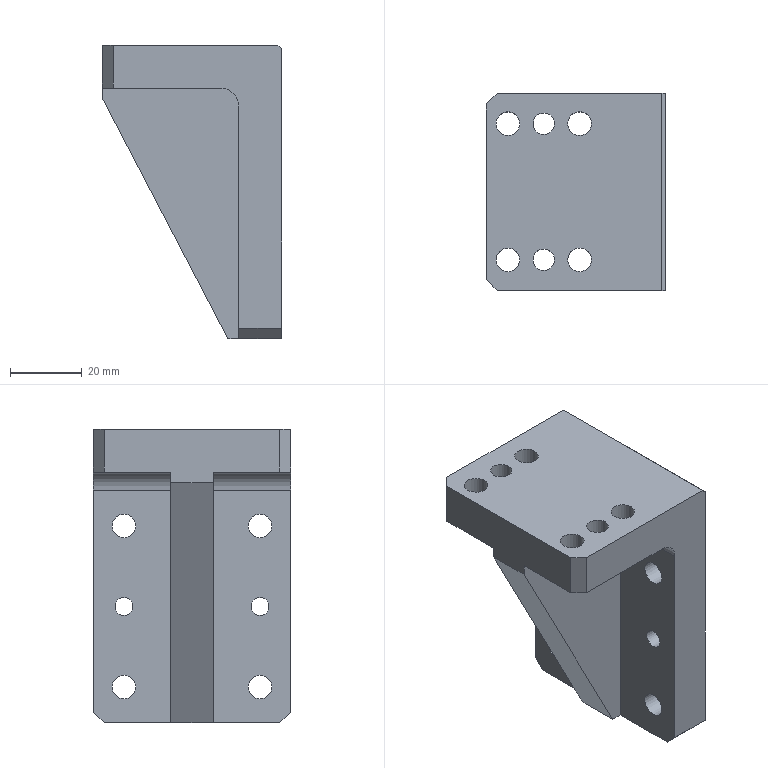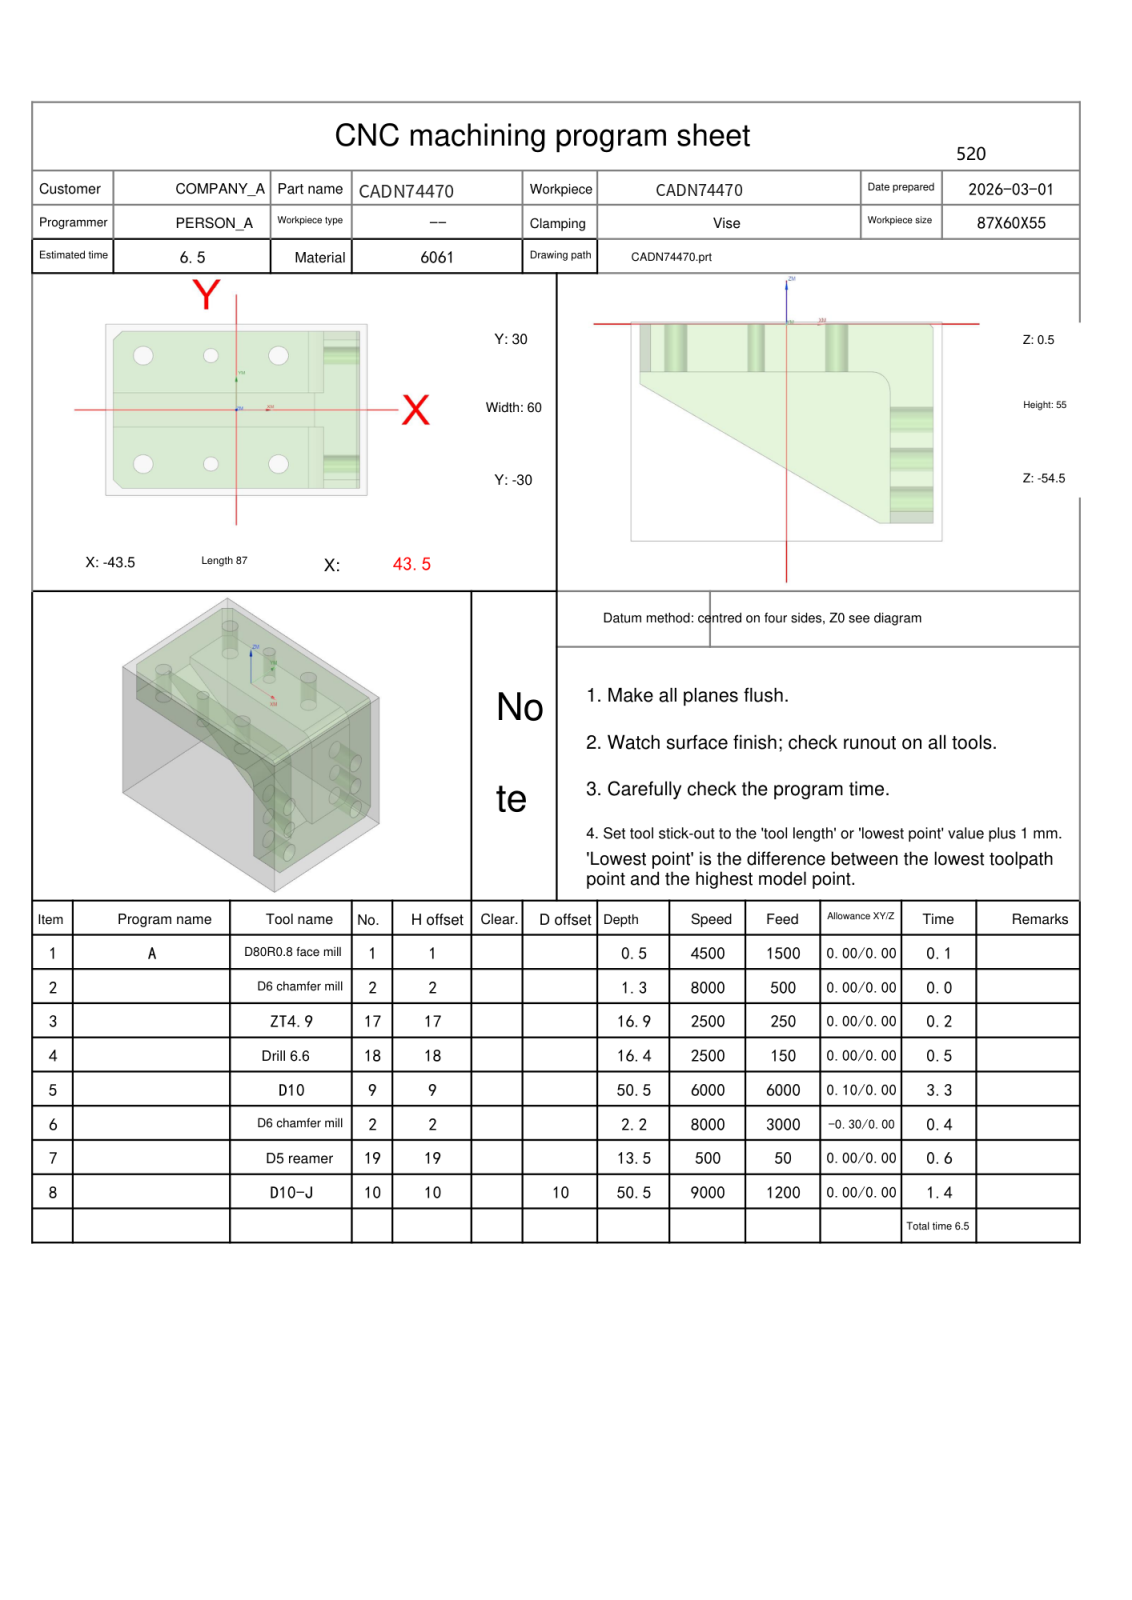NC program | NX | posted by the shop | part box 50 x 55 x 82 mm
Whole program:
%
O0001
(Machine time: 7.98 MIN)
(===Total Tool:7===)
(T1=D80R0.8 face mill D=80.  R=0.8  D-  H01 Z=-0.   )
(T2=D6 chamfer mill   D=6.   R=0.   D-  H02 Z=-1.7  )
(T17=ZT4.9  D=4.9  DR_a=120 D-  H17 Z=-16.41)
(T18=drill 6.6  D=6.6  DR_a=120 D-  H18 Z=-15.91)
(T9=D10     D=10.  R=0.   D-  H09 Z=-50.  )
(T19=D5 reamer   D=5.   DR_a=180 D-  H19 Z=-13.  )
(T10=D10-J  D=10.  R=0.   D10 H10 Z=-50.  )
G80 G90 G17 G49 G40
G91 G28 Z0
M01
N1 T01 M06
(D80R0.8 face mill  D=80. R=0.8 H=01 ce=0.00 di=0.00)
G00 G90 G54 X86. Y0.0 M03 S4500
G43 H01 Z50.
M08
Z2.
G01 Z0.0 F1500.
X81.
X-81.
X-86.
Z2.
G00 Z50.
G91 G28 Z0.0
M05
M09
G91 G28 Z0.0
M01
N2 T02 M06
(D6 chamfer mill  D=6. R=0. H=02 ce=0.00 di=0.00)
G00 G90 G54 X14. Y-19. M03 S8000
G43 H02 Z50.
M08
G98 G81 X14. Y-19. Z-.8 R1. F500.
X-8.5
X-31.
Y19.
X-8.5
X14.
G80
G00 Z50.
G91 G28 Z0.0
M05
M09
G91 G28 Z0.0
M01
N3 T17 M06
(ZT4.9 D=4.9 DR_a=120 H=17)
G00 G90 G54 X-8.5 Y-19. M03 S2500
G43 H17 Z50.
M08
G98 G83 X-8.5 Y-19. Z-16.415 R1. F250. Q2.
Y19.
G80
G00 Z50.
G91 G28 Z0.0
M05
M09
G91 G28 Z0.0
M01
N4 T18 M06
(drill 6.6 D=6.6 DR_a=120 H=18)
G00 G90 G54 X14. Y-19. M03 S2500
G43 H18 Z50.
M08
G98 G83 X14. Y-19. Z-15.905 R1. F150. Q3.
Y19.
X-31.
Y-19.
G80
G00 Z50.
G91 G28 Z0.0
M05
M09
G91 G28 Z0.0
M01
N5 T09 M06
(D10  D=10. R=0. H=09 ce=0.10 di=0.00)
G00 G90 G54 X1.081 Y-32.6 M03 S6000
G43 H09 Z50.
M08
Z.5
G01 X-38. Z.398 F6000.
G02 X-38.835 Y-32.531 Z.396 I0.0 J5.1
X-41.606 Y-31.106 Z.388 I.835 J5.031
G01 X-44.606 Y-28.106 Z.377
G02 X-46.1 Y-24.5 Z.366 I3.606 J3.606
G01 Y24.5 Z.238
G02 X-44.606 Y28.106 Z.228 I5.1 J0.0
G01 X-41.606 Y31.106 Z.217
G02 X-38. Y32.6 Z.206 I3.606 J-3.606
G01 X41. Z0.0
G02 X46.1 Y27.5 Z-.021 I0.0 J-5.1
G01 Y-27.5 Z-.164
G02 X41. Y-32.6 Z-.185 I-5.1 J0.0
G01 X-38. Z-.391
G02 X-38.835 Y-32.531 Z-.393 I0.0 J5.1
X-41.606 Y-31.106 Z-.401 I.835 J5.031
G01 X-44.606 Y-28.106 Z-.413
G02 X-46.1 Y-24.5 Z-.423 I3.606 J3.606
G01 Y24.5 Z-.551
G02 X-44.606 Y28.106 Z-.561 I5.1 J0.0
G01 X-41.606 Y31.106 Z-.572
G02 X-38. Y32.6 Z-.583 I3.606 J-3.606
G01 X41. Z-.789
G02 X46.1 Y27.5 Z-.81 I0.0 J-5.1
G01 Y-27.5 Z-.953
G02 X41. Y-32.6 Z-.974 I-5.1 J0.0
G01 X-38. Z-1.18
G02 X-38.835 Y-32.531 Z-1.182 I0.0 J5.1
X-41.606 Y-31.106 Z-1.191 I.835 J5.031
G01 X-44.606 Y-28.106 Z-1.202
G02 X-46.1 Y-24.5 Z-1.212 I3.606 J3.606
G01 Y24.5 Z-1.34
G02 X-44.606 Y28.106 Z-1.35 I5.1 J0.0
G01 X-41.606 Y31.106 Z-1.361
G02 X-38. Y32.6 Z-1.372 I3.606 J-3.606
G01 X41. Z-1.578
G02 X46.1 Y27.5 Z-1.599 I0.0 J-5.1
G01 Y-27.5 Z-1.742
G02 X41. Y-32.6 Z-1.763 I-5.1 J0.0
G01 X-38. Z-1.969
G02 X-38.835 Y-32.531 Z-1.971 I0.0 J5.1
X-41.606 Y-31.106 Z-1.98 I.835 J5.031
G01 X-44.606 Y-28.106 Z-1.991
G02 X-46.1 Y-24.5 Z-2.001 I3.606 J3.606
G01 Y24.5 Z-2.129
G02 X-44.606 Y28.106 Z-2.139 I5.1 J0.0
G01 X-41.606 Y31.106 Z-2.15
G02 X-38. Y32.6 Z-2.161 I3.606 J-3.606
G01 X41. Z-2.367
G02 X46.1 Y27.5 Z-2.388 I0.0 J-5.1
G01 Y-27.5 Z-2.531
G02 X41. Y-32.6 Z-2.552 I-5.1 J0.0
G01 X-38. Z-2.758
G02 X-38.835 Y-32.531 Z-2.76 I0.0 J5.1
X-41.606 Y-31.106 Z-2.769 I.835 J5.031
G01 X-44.606 Y-28.106 Z-2.78
G02 X-46.1 Y-24.5 Z-2.79 I3.606 J3.606
G01 Y24.5 Z-2.918
G02 X-44.606 Y28.106 Z-2.928 I5.1 J0.0
G01 X-41.606 Y31.106 Z-2.939
G02 X-38. Y32.6 Z-2.95 I3.606 J-3.606
G01 X41. Z-3.156
G02 X46.1 Y27.5 Z-3.177 I0.0 J-5.1
G01 Y-27.5 Z-3.32
G02 X41. Y-32.6 Z-3.341 I-5.1 J0.0
G01 X-38. Z-3.547
G02 X-38.835 Y-32.531 Z-3.549 I0.0 J5.1
X-41.606 Y-31.106 Z-3.558 I.835 J5.031
G01 X-44.606 Y-28.106 Z-3.569
G02 X-46.1 Y-24.5 Z-3.579 I3.606 J3.606
G01 Y24.5 Z-3.707
G02 X-44.606 Y28.106 Z-3.717 I5.1 J0.0
G01 X-41.606 Y31.106 Z-3.729
G02 X-38. Y32.6 Z-3.739 I3.606 J-3.606
G01 X41. Z-3.945
G02 X46.1 Y27.5 Z-3.966 I0.0 J-5.1
G01 Y-27.5 Z-4.109
G02 X41. Y-32.6 Z-4.13 I-5.1 J0.0
G01 X-38. Z-4.336
G02 X-38.835 Y-32.531 Z-4.338 I0.0 J5.1
X-41.606 Y-31.106 Z-4.347 I.835 J5.031
G01 X-44.606 Y-28.106 Z-4.358
G02 X-46.1 Y-24.5 Z-4.368 I3.606 J3.606
G01 Y24.5 Z-4.496
G02 X-44.606 Y28.106 Z-4.507 I5.1 J0.0
G01 X-41.606 Y31.106 Z-4.518
G02 X-38. Y32.6 Z-4.528 I3.606 J-3.606
G01 X41. Z-4.734
G02 X46.1 Y27.5 Z-4.755 I0.0 J-5.1
G01 Y-27.5 Z-4.898
G02 X41. Y-32.6 Z-4.919 I-5.1 J0.0
G01 X-38. Z-5.125
G02 X-38.835 Y-32.531 Z-5.128 I0.0 J5.1
X-41.606 Y-31.106 Z-5.136 I.835 J5.031
G01 X-44.606 Y-28.106 Z-5.147
G02 X-46.1 Y-24.5 Z-5.157 I3.606 J3.606
G01 Y24.5 Z-5.285
G02 X-44.606 Y28.106 Z-5.296 I5.1 J0.0
G01 X-41.606 Y31.106 Z-5.307
G02 X-38. Y32.6 Z-5.317 I3.606 J-3.606
G01 X41. Z-5.523
G02 X46.1 Y27.5 Z-5.544 I0.0 J-5.1
G01 Y-27.5 Z-5.687
G02 X41. Y-32.6 Z-5.708 I-5.1 J0.0
G01 X-38. Z-5.914
G02 X-38.835 Y-32.531 Z-5.917 I0.0 J5.1
X-41.606 Y-31.106 Z-5.925 I.835 J5.031
G01 X-44.606 Y-28.106 Z-5.936
G02 X-46.1 Y-24.5 Z-5.946 I3.606 J3.606
G01 Y24.5 Z-6.074
G02 X-44.606 Y28.106 Z-6.085 I5.1 J0.0
G01 X-41.606 Y31.106 Z-6.096
G02 X-38. Y32.6 Z-6.106 I3.606 J-3.606
G01 X41. Z-6.312
G02 X46.1 Y27.5 Z-6.333 I0.0 J-5.1
G01 Y-27.5 Z-6.477
G02 X41. Y-32.6 Z-6.497 I-5.1 J0.0
G01 X-38. Z-6.703
G02 X-38.835 Y-32.531 Z-6.706 I0.0 J5.1
X-41.606 Y-31.106 Z-6.714 I.835 J5.031
G01 X-44.606 Y-28.106 Z-6.725
G02 X-46.1 Y-24.5 Z-6.735 I3.606 J3.606
G01 Y24.5 Z-6.863
G02 X-44.606 Y28.106 Z-6.874 I5.1 J0.0
G01 X-41.606 Y31.106 Z-6.885
G02 X-38. Y32.6 Z-6.895 I3.606 J-3.606
G01 X41. Z-7.101
G02 X46.1 Y27.5 Z-7.122 I0.0 J-5.1
G01 Y-27.5 Z-7.266
G02 X41. Y-32.6 Z-7.287 I-5.1 J0.0
G01 X-38. Z-7.493
G02 X-38.835 Y-32.531 Z-7.495 I0.0 J5.1
X-41.606 Y-31.106 Z-7.503 I.835 J5.031
G01 X-44.606 Y-28.106 Z-7.514
G02 X-46.1 Y-24.5 Z-7.525 I3.606 J3.606
G01 Y24.5 Z-7.652
G02 X-44.606 Y28.106 Z-7.663 I5.1 J0.0
G01 X-41.606 Y31.106 Z-7.674
G02 X-38. Y32.6 Z-7.684 I3.606 J-3.606
G01 X41. Z-7.89
G02 X46.1 Y27.5 Z-7.911 I0.0 J-5.1
G01 Y-27.5 Z-8.055
G02 X41. Y-32.6 Z-8.076 I-5.1 J0.0
G01 X-38. Z-8.282
G02 X-38.835 Y-32.531 Z-8.284 I0.0 J5.1
X-41.606 Y-31.106 Z-8.292 I.835 J5.031
G01 X-44.606 Y-28.106 Z-8.303
G02 X-46.1 Y-24.5 Z-8.314 I3.606 J3.606
G01 Y24.5 Z-8.441
G02 X-44.606 Y28.106 Z-8.452 I5.1 J0.0
G01 X-41.606 Y31.106 Z-8.463
G02 X-38. Y32.6 Z-8.473 I3.606 J-3.606
G01 X41. Z-8.679
G02 X46.1 Y27.5 Z-8.7 I0.0 J-5.1
G01 Y-27.5 Z-8.844
G02 X41. Y-32.6 Z-8.865 I-5.1 J0.0
G01 X-38. Z-9.071
G02 X-38.835 Y-32.531 Z-9.073 I0.0 J5.1
X-41.606 Y-31.106 Z-9.081 I.835 J5.031
G01 X-44.606 Y-28.106 Z-9.092
G02 X-46.1 Y-24.5 Z-9.103 I3.606 J3.606
G01 Y24.5 Z-9.23
G02 X-44.606 Y28.106 Z-9.241 I5.1 J0.0
G01 X-41.606 Y31.106 Z-9.252
G02 X-38. Y32.6 Z-9.262 I3.606 J-3.606
G01 X41. Z-9.468
G02 X46.1 Y27.5 Z-9.489 I0.0 J-5.1
G01 Y-27.5 Z-9.633
G02 X41. Y-32.6 Z-9.654 I-5.1 J0.0
G01 X-38. Z-9.86
G02 X-38.835 Y-32.531 Z-9.862 I0.0 J5.1
X-41.606 Y-31.106 Z-9.87 I.835 J5.031
G01 X-44.606 Y-28.106 Z-9.881
G02 X-46.1 Y-24.5 Z-9.892 I3.606 J3.606
G01 Y24.5 Z-10.02
G02 X-44.606 Y28.106 Z-10.03 I5.1 J0.0
G01 X-41.606 Y31.106 Z-10.041
G02 X-38. Y32.6 Z-10.051 I3.606 J-3.606
G01 X41. Z-10.258
G02 X46.1 Y27.5 Z-10.278 I0.0 J-5.1
G01 Y-27.5 Z-10.422
G02 X41. Y-32.6 Z-10.443 I-5.1 J0.0
G01 X-38. Z-10.649
G02 X-38.835 Y-32.531 Z-10.651 I0.0 J5.1
X-41.606 Y-31.106 Z-10.659 I.835 J5.031
G01 X-44.606 Y-28.106 Z-10.67
G02 X-46.1 Y-24.5 Z-10.681 I3.606 J3.606
G01 Y24.5 Z-10.809
G02 X-44.606 Y28.106 Z-10.819 I5.1 J0.0
G01 X-41.606 Y31.106 Z-10.83
G02 X-38. Y32.6 Z-10.841 I3.606 J-3.606
G01 X41. Z-11.047
G02 X46.1 Y27.5 Z-11.067 I0.0 J-5.1
G01 Y-27.5 Z-11.211
G02 X41. Y-32.6 Z-11.232 I-5.1 J0.0
G01 X-38. Z-11.438
G02 X-38.835 Y-32.531 Z-11.44 I0.0 J5.1
X-41.606 Y-31.106 Z-11.448 I.835 J5.031
G01 X-44.606 Y-28.106 Z-11.459
G02 X-46.1 Y-24.5 Z-11.47 I3.606 J3.606
G01 Y24.5 Z-11.598
G02 X-44.606 Y28.106 Z-11.608 I5.1 J0.0
G01 X-41.606 Y31.106 Z-11.619
G02 X-38. Y32.6 Z-11.63 I3.606 J-3.606
G01 X41. Z-11.836
G02 X46.1 Y27.5 Z-11.857 I0.0 J-5.1
G01 Y-27.5 Z-12.
G02 X41. Y-32.6 Z-12.021 I-5.1 J0.0
G01 X-38. Z-12.227
G02 X-38.835 Y-32.531 Z-12.229 I0.0 J5.1
X-41.606 Y-31.106 Z-12.237 I.835 J5.031
G01 X-44.606 Y-28.106 Z-12.248
G02 X-46.1 Y-24.5 Z-12.259 I3.606 J3.606
G01 Y24.5 Z-12.387
G02 X-44.606 Y28.106 Z-12.397 I5.1 J0.0
G01 X-41.606 Y31.106 Z-12.408
G02 X-38. Y32.6 Z-12.419 I3.606 J-3.606
G01 X41. Z-12.625
G02 X46.1 Y27.5 Z-12.646 I0.0 J-5.1
G01 Y-27.5 Z-12.789
G02 X41. Y-32.6 Z-12.81 I-5.1 J0.0
G01 X-38. Z-13.016
G02 X-38.835 Y-32.531 Z-13.018 I0.0 J5.1
X-41.606 Y-31.106 Z-13.026 I.835 J5.031
G01 X-44.606 Y-28.106 Z-13.038
G02 X-46.1 Y-24.5 Z-13.048 I3.606 J3.606
G01 Y24.5 Z-13.176
G02 X-44.606 Y28.106 Z-13.186 I5.1 J0.0
G01 X-41.606 Y31.106 Z-13.197
G02 X-38. Y32.6 Z-13.208 I3.606 J-3.606
G01 X41. Z-13.414
G02 X46.1 Y27.5 Z-13.435 I0.0 J-5.1
G01 Y-27.5 Z-13.578
G02 X41. Y-32.6 Z-13.599 I-5.1 J0.0
G01 X-38. Z-13.805
G02 X-38.835 Y-32.531 Z-13.807 I0.0 J5.1
X-41.606 Y-31.106 Z-13.816 I.835 J5.031
G01 X-44.606 Y-28.106 Z-13.827
G02 X-46.1 Y-24.5 Z-13.837 I3.606 J3.606
G01 Y24.5 Z-13.965
G02 X-44.606 Y28.106 Z-13.975 I5.1 J0.0
G01 X-41.606 Y31.106 Z-13.986
G02 X-38. Y32.6 Z-13.997 I3.606 J-3.606
G01 X41. Z-14.203
G02 X46.1 Y27.5 Z-14.224 I0.0 J-5.1
G01 Y-27.5 Z-14.367
G02 X41. Y-32.6 Z-14.388 I-5.1 J0.0
G01 X-38. Z-14.594
G02 X-38.835 Y-32.531 Z-14.596 I0.0 J5.1
X-41.606 Y-31.106 Z-14.605 I.835 J5.031
G01 X-44.606 Y-28.106 Z-14.616
G02 X-46.1 Y-24.5 Z-14.626 I3.606 J3.606
G01 Y24.5 Z-14.754
G02 X-44.606 Y28.106 Z-14.764 I5.1 J0.0
G01 X-41.606 Y31.106 Z-14.775
G02 X-38. Y32.6 Z-14.786 I3.606 J-3.606
G01 X41. Z-14.992
G02 X46.1 Y27.5 Z-15.013 I0.0 J-5.1
G01 Y-27.5 Z-15.156
G02 X41. Y-32.6 Z-15.177 I-5.1 J0.0
G01 X-38. Z-15.383
G02 X-38.835 Y-32.531 Z-15.385 I0.0 J5.1
X-41.606 Y-31.106 Z-15.394 I.835 J5.031
G01 X-44.606 Y-28.106 Z-15.405
G02 X-46.1 Y-24.5 Z-15.415 I3.606 J3.606
G01 Y24.5 Z-15.543
G02 X-44.606 Y28.106 Z-15.553 I5.1 J0.0
G01 X-41.606 Y31.106 Z-15.564
G02 X-38. Y32.6 Z-15.575 I3.606 J-3.606
G01 X41. Z-15.781
G02 X46.1 Y27.5 Z-15.802 I0.0 J-5.1
G01 Y-27.5 Z-15.945
G02 X41. Y-32.6 Z-15.966 I-5.1 J0.0
G01 X-38. Z-16.172
G02 X-38.835 Y-32.531 Z-16.174 I0.0 J5.1
X-41.606 Y-31.106 Z-16.183 I.835 J5.031
G01 X-44.606 Y-28.106 Z-16.194
G02 X-46.1 Y-24.5 Z-16.204 I3.606 J3.606
G01 Y24.5 Z-16.332
G02 X-44.606 Y28.106 Z-16.342 I5.1 J0.0
G01 X-41.606 Y31.106 Z-16.354
G02 X-38. Y32.6 Z-16.364 I3.606 J-3.606
G01 X41. Z-16.57
G02 X46.1 Y27.5 Z-16.591 I0.0 J-5.1
G01 Y-27.5 Z-16.734
G02 X41. Y-32.6 Z-16.755 I-5.1 J0.0
G01 X-38. Z-16.961
G02 X-38.835 Y-32.531 Z-16.963 I0.0 J5.1
X-41.606 Y-31.106 Z-16.972 I.835 J5.031
G01 X-44.606 Y-28.106 Z-16.983
G02 X-46.1 Y-24.5 Z-16.993 I3.606 J3.606
G01 Y24.5 Z-17.121
G02 X-44.606 Y28.106 Z-17.132 I5.1 J0.0
G01 X-41.606 Y31.106 Z-17.143
G02 X-38. Y32.6 Z-17.153 I3.606 J-3.606
G01 X41. Z-17.359
G02 X46.1 Y27.5 Z-17.38 I0.0 J-5.1
G01 Y-27.5 Z-17.523
G02 X41. Y-32.6 Z-17.544 I-5.1 J0.0
G01 X-38. Z-17.75
G02 X-38.835 Y-32.531 Z-17.753 I0.0 J5.1
X-41.606 Y-31.106 Z-17.761 I.835 J5.031
G01 X-44.606 Y-28.106 Z-17.772
G02 X-46.1 Y-24.5 Z-17.782 I3.606 J3.606
G01 Y24.5 Z-17.91
G02 X-44.606 Y28.106 Z-17.921 I5.1 J0.0
G01 X-41.606 Y31.106 Z-17.932
G02 X-38. Y32.6 Z-17.942 I3.606 J-3.606
G01 X41. Z-18.148
G02 X46.1 Y27.5 Z-18.169 I0.0 J-5.1
G01 Y-27.5 Z-18.312
G02 X41. Y-32.6 Z-18.333 I-5.1 J0.0
G01 X-38. Z-18.539
G02 X-38.835 Y-32.531 Z-18.542 I0.0 J5.1
X-41.606 Y-31.106 Z-18.55 I.835 J5.031
G01 X-44.606 Y-28.106 Z-18.561
G02 X-46.1 Y-24.5 Z-18.571 I3.606 J3.606
G01 Y24.5 Z-18.699
G02 X-44.606 Y28.106 Z-18.71 I5.1 J0.0
G01 X-41.606 Y31.106 Z-18.721
G02 X-38. Y32.6 Z-18.731 I3.606 J-3.606
G01 X41. Z-18.937
G02 X46.1 Y27.5 Z-18.958 I0.0 J-5.1
G01 Y-27.5 Z-19.102
G02 X41. Y-32.6 Z-19.122 I-5.1 J0.0
G01 X-38. Z-19.328
G02 X-38.835 Y-32.531 Z-19.331 I0.0 J5.1
X-41.606 Y-31.106 Z-19.339 I.835 J5.031
G01 X-44.606 Y-28.106 Z-19.35
G02 X-46.1 Y-24.5 Z-19.36 I3.606 J3.606
G01 Y24.5 Z-19.488
G02 X-44.606 Y28.106 Z-19.499 I5.1 J0.0
G01 X-41.606 Y31.106 Z-19.51
G02 X-38. Y32.6 Z-19.52 I3.606 J-3.606
G01 X41. Z-19.726
G02 X46.1 Y27.5 Z-19.747 I0.0 J-5.1
G01 Y-27.5 Z-19.891
G02 X41. Y-32.6 Z-19.912 I-5.1 J0.0
G01 X-38. Z-20.118
G02 X-38.835 Y-32.531 Z-20.12 I0.0 J5.1
X-41.606 Y-31.106 Z-20.128 I.835 J5.031
G01 X-44.606 Y-28.106 Z-20.139
G02 X-46.1 Y-24.5 Z-20.15 I3.606 J3.606
G01 Y24.5 Z-20.277
G02 X-44.606 Y28.106 Z-20.288 I5.1 J0.0
G01 X-41.606 Y31.106 Z-20.299
G02 X-38. Y32.6 Z-20.309 I3.606 J-3.606
G01 X41. Z-20.515
G02 X46.1 Y27.5 Z-20.536 I0.0 J-5.1
G01 Y-27.5 Z-20.68
G02 X41. Y-32.6 Z-20.701 I-5.1 J0.0
G01 X-38. Z-20.907
G02 X-38.835 Y-32.531 Z-20.909 I0.0 J5.1
X-41.606 Y-31.106 Z-20.917 I.835 J5.031
G01 X-44.606 Y-28.106 Z-20.928
G02 X-46.1 Y-24.5 Z-20.939 I3.606 J3.606
G01 Y24.5 Z-21.066
G02 X-44.606 Y28.106 Z-21.077 I5.1 J0.0
G01 X-41.606 Y31.106 Z-21.088
G02 X-38. Y32.6 Z-21.098 I3.606 J-3.606
G01 X41. Z-21.304
G02 X46.1 Y27.5 Z-21.325 I0.0 J-5.1
G01 Y-27.5 Z-21.469
G02 X41. Y-32.6 Z-21.49 I-5.1 J0.0
G01 X-38. Z-21.696
G02 X-38.835 Y-32.531 Z-21.698 I0.0 J5.1
X-41.606 Y-31.106 Z-21.706 I.835 J5.031
G01 X-44.606 Y-28.106 Z-21.717
G02 X-46.1 Y-24.5 Z-21.728 I3.606 J3.606
G01 Y24.5 Z-21.855
G02 X-44.606 Y28.106 Z-21.866 I5.1 J0.0
G01 X-41.606 Y31.106 Z-21.877
G02 X-38. Y32.6 Z-21.887 I3.606 J-3.606
G01 X41. Z-22.093
G02 X46.1 Y27.5 Z-22.114 I0.0 J-5.1
G01 Y-27.5 Z-22.258
G02 X41. Y-32.6 Z-22.279 I-5.1 J0.0
G01 X-38. Z-22.485
G02 X-38.835 Y-32.531 Z-22.487 I0.0 J5.1
X-41.606 Y-31.106 Z-22.495 I.835 J5.031
G01 X-44.606 Y-28.106 Z-22.506
G02 X-46.1 Y-24.5 Z-22.517 I3.606 J3.606
G01 Y24.5 Z-22.645
G02 X-44.606 Y28.106 Z-22.655 I5.1 J0.0
G01 X-41.606 Y31.106 Z-22.666
G02 X-38. Y32.6 Z-22.676 I3.606 J-3.606
G01 X41. Z-22.883
G02 X46.1 Y27.5 Z-22.903 I0.0 J-5.1
G01 Y-27.5 Z-23.047
G02 X41. Y-32.6 Z-23.068 I-5.1 J0.0
G01 X-38. Z-23.274
G02 X-38.835 Y-32.531 Z-23.276 I0.0 J5.1
X-41.606 Y-31.106 Z-23.284 I.835 J5.031
G01 X-44.606 Y-28.106 Z-23.295
G02 X-46.1 Y-24.5 Z-23.306 I3.606 J3.606
G01 Y24.5 Z-23.434
G02 X-44.606 Y28.106 Z-23.444 I5.1 J0.0
G01 X-41.606 Y31.106 Z-23.455
G02 X-38. Y32.6 Z-23.466 I3.606 J-3.606
G01 X41. Z-23.672
G02 X46.1 Y27.5 Z-23.692 I0.0 J-5.1
G01 Y-27.5 Z-23.836
G02 X41. Y-32.6 Z-23.857 I-5.1 J0.0
G01 X-38. Z-24.063
G02 X-38.835 Y-32.531 Z-24.065 I0.0 J5.1
X-41.606 Y-31.106 Z-24.073 I.835 J5.031
G01 X-44.606 Y-28.106 Z-24.084
G02 X-46.1 Y-24.5 Z-24.095 I3.606 J3.606
G01 Y24.5 Z-24.223
G02 X-44.606 Y28.106 Z-24.233 I5.1 J0.0
G01 X-41.606 Y31.106 Z-24.244
G02 X-38. Y32.6 Z-24.255 I3.606 J-3.606
G01 X41. Z-24.461
G02 X46.1 Y27.5 Z-24.482 I0.0 J-5.1
G01 Y-27.5 Z-24.625
G02 X41. Y-32.6 Z-24.646 I-5.1 J0.0
G01 X-38. Z-24.852
G02 X-38.835 Y-32.531 Z-24.854 I0.0 J5.1
X-41.606 Y-31.106 Z-24.862 I.835 J5.031
G01 X-44.606 Y-28.106 Z-24.873
G02 X-46.1 Y-24.5 Z-24.884 I3.606 J3.606
G01 Y24.5 Z-25.012
G02 X-44.606 Y28.106 Z-25.022 I5.1 J0.0
G01 X-41.606 Y31.106 Z-25.033
G02 X-38. Y32.6 Z-25.044 I3.606 J-3.606
G01 X41. Z-25.25
G02 X46.1 Y27.5 Z-25.271 I0.0 J-5.1
G01 Y-27.5 Z-25.414
G02 X41. Y-32.6 Z-25.435 I-5.1 J0.0
G01 X-38. Z-25.641
G02 X-38.835 Y-32.531 Z-25.643 I0.0 J5.1
X-41.606 Y-31.106 Z-25.651 I.835 J5.031
G01 X-44.606 Y-28.106 Z-25.663
G02 X-46.1 Y-24.5 Z-25.673 I3.606 J3.606
G01 Y24.5 Z-25.801
G02 X-44.606 Y28.106 Z-25.811 I5.1 J0.0
G01 X-41.606 Y31.106 Z-25.822
G02 X-38. Y32.6 Z-25.833 I3.606 J-3.606
G01 X41. Z-26.039
G02 X46.1 Y27.5 Z-26.06 I0.0 J-5.1
G01 Y-27.5 Z-26.203
G02 X41. Y-32.6 Z-26.224 I-5.1 J0.0
G01 X-38. Z-26.43
G02 X-38.835 Y-32.531 Z-26.432 I0.0 J5.1
X-41.606 Y-31.106 Z-26.441 I.835 J5.031
G01 X-44.606 Y-28.106 Z-26.452
G02 X-46.1 Y-24.5 Z-26.462 I3.606 J3.606
G01 Y24.5 Z-26.59
G02 X-44.606 Y28.106 Z-26.6 I5.1 J0.0
G01 X-41.606 Y31.106 Z-26.611
G02 X-38. Y32.6 Z-26.622 I3.606 J-3.606
G01 X41. Z-26.828
G02 X46.1 Y27.5 Z-26.849 I0.0 J-5.1
G01 Y-27.5 Z-26.992
G02 X41. Y-32.6 Z-27.013 I-5.1 J0.0
G01 X-38. Z-27.219
G02 X-38.835 Y-32.531 Z-27.221 I0.0 J5.1
X-41.606 Y-31.106 Z-27.23 I.835 J5.031
G01 X-44.606 Y-28.106 Z-27.241
G02 X-46.1 Y-24.5 Z-27.251 I3.606 J3.606
G01 Y24.5 Z-27.379
G02 X-44.606 Y28.106 Z-27.389 I5.1 J0.0
G01 X-41.606 Y31.106 Z-27.4
G02 X-38. Y32.6 Z-27.411 I3.606 J-3.606
G01 X41. Z-27.617
G02 X46.1 Y27.5 Z-27.638 I0.0 J-5.1
G01 Y-27.5 Z-27.781
G02 X41. Y-32.6 Z-27.802 I-5.1 J0.0
G01 X-38. Z-28.008
G02 X-38.835 Y-32.531 Z-28.01 I0.0 J5.1
X-41.606 Y-31.106 Z-28.019 I.835 J5.031
G01 X-44.606 Y-28.106 Z-28.03
G02 X-46.1 Y-24.5 Z-28.04 I3.606 J3.606
G01 Y24.5 Z-28.168
G02 X-44.606 Y28.106 Z-28.178 I5.1 J0.0
G01 X-41.606 Y31.106 Z-28.189
G02 X-38. Y32.6 Z-28.2 I3.606 J-3.606
G01 X41. Z-28.406
G02 X46.1 Y27.5 Z-28.427 I0.0 J-5.1
G01 Y-27.5 Z-28.57
G02 X41. Y-32.6 Z-28.591 I-5.1 J0.0
G01 X-38. Z-28.797
G02 X-38.835 Y-32.531 Z-28.799 I0.0 J5.1
X-41.606 Y-31.106 Z-28.808 I.835 J5.031
G01 X-44.606 Y-28.106 Z-28.819
G02 X-46.1 Y-24.5 Z-28.829 I3.606 J3.606
G01 Y24.5 Z-28.957
G02 X-44.606 Y28.106 Z-28.967 I5.1 J0.0
G01 X-41.606 Y31.106 Z-28.979
G02 X-38. Y32.6 Z-28.989 I3.606 J-3.606
G01 X41. Z-29.195
G02 X46.1 Y27.5 Z-29.216 I0.0 J-5.1
G01 Y-27.5 Z-29.359
G02 X41. Y-32.6 Z-29.38 I-5.1 J0.0
G01 X-38. Z-29.586
G02 X-38.835 Y-32.531 Z-29.588 I0.0 J5.1
X-41.606 Y-31.106 Z-29.597 I.835 J5.031
G01 X-44.606 Y-28.106 Z-29.608
G02 X-46.1 Y-24.5 Z-29.618 I3.606 J3.606
G01 Y24.5 Z-29.746
G02 X-44.606 Y28.106 Z-29.757 I5.1 J0.0
G01 X-41.606 Y31.106 Z-29.768
G02 X-38. Y32.6 Z-29.778 I3.606 J-3.606
G01 X41. Z-29.984
G02 X46.1 Y27.5 Z-30.005 I0.0 J-5.1
G01 Y-27.5 Z-30.148
G02 X41. Y-32.6 Z-30.169 I-5.1 J0.0
G01 X-38. Z-30.375
G02 X-38.835 Y-32.531 Z-30.378 I0.0 J5.1
X-41.606 Y-31.106 Z-30.386 I.835 J5.031
G01 X-44.606 Y-28.106 Z-30.397
G02 X-46.1 Y-24.5 Z-30.407 I3.606 J3.606
G01 Y24.5 Z-30.535
G02 X-44.606 Y28.106 Z-30.546 I5.1 J0.0
G01 X-41.606 Y31.106 Z-30.557
G02 X-38. Y32.6 Z-30.567 I3.606 J-3.606
G01 X41. Z-30.773
G02 X46.1 Y27.5 Z-30.794 I0.0 J-5.1
G01 Y-27.5 Z-30.937
G02 X41. Y-32.6 Z-30.958 I-5.1 J0.0
G01 X-38. Z-31.164
G02 X-38.835 Y-32.531 Z-31.167 I0.0 J5.1
X-41.606 Y-31.106 Z-31.175 I.835 J5.031
G01 X-44.606 Y-28.106 Z-31.186
G02 X-46.1 Y-24.5 Z-31.196 I3.606 J3.606
G01 Y24.5 Z-31.324
G02 X-44.606 Y28.106 Z-31.335 I5.1 J0.0
G01 X-41.606 Y31.106 Z-31.346
G02 X-38. Y32.6 Z-31.356 I3.606 J-3.606
G01 X41. Z-31.562
G02 X46.1 Y27.5 Z-31.583 I0.0 J-5.1
G01 Y-27.5 Z-31.727
G02 X41. Y-32.6 Z-31.747 I-5.1 J0.0
G01 X-38. Z-31.953
G02 X-38.835 Y-32.531 Z-31.956 I0.0 J5.1
X-41.606 Y-31.106 Z-31.964 I.835 J5.031
G01 X-44.606 Y-28.106 Z-31.975
G02 X-46.1 Y-24.5 Z-31.985 I3.606 J3.606
G01 Y24.5 Z-32.113
G02 X-44.606 Y28.106 Z-32.124 I5.1 J0.0
G01 X-41.606 Y31.106 Z-32.135
G02 X-38. Y32.6 Z-32.145 I3.606 J-3.606
G01 X41. Z-32.351
G02 X46.1 Y27.5 Z-32.372 I0.0 J-5.1
G01 Y-27.5 Z-32.516
G02 X41. Y-32.6 Z-32.537 I-5.1 J0.0
G01 X-38. Z-32.743
G02 X-38.835 Y-32.531 Z-32.745 I0.0 J5.1
X-41.606 Y-31.106 Z-32.753 I.835 J5.031
G01 X-44.606 Y-28.106 Z-32.764
G02 X-46.1 Y-24.5 Z-32.775 I3.606 J3.606
G01 Y24.5 Z-32.902
G02 X-44.606 Y28.106 Z-32.913 I5.1 J0.0
G01 X-41.606 Y31.106 Z-32.924
G02 X-38. Y32.6 Z-32.934 I3.606 J-3.606
G01 X41. Z-33.14
G02 X46.1 Y27.5 Z-33.161 I0.0 J-5.1
G01 Y-27.5 Z-33.305
G02 X41. Y-32.6 Z-33.326 I-5.1 J0.0
G01 X-38. Z-33.532
G02 X-38.835 Y-32.531 Z-33.534 I0.0 J5.1
X-41.606 Y-31.106 Z-33.542 I.835 J5.031
G01 X-44.606 Y-28.106 Z-33.553
G02 X-46.1 Y-24.5 Z-33.564 I3.606 J3.606
G01 Y24.5 Z-33.691
G02 X-44.606 Y28.106 Z-33.702 I5.1 J0.0
G01 X-41.606 Y31.106 Z-33.713
G02 X-38. Y32.6 Z-33.723 I3.606 J-3.606
G01 X41. Z-33.929
G02 X46.1 Y27.5 Z-33.95 I0.0 J-5.1
G01 Y-27.5 Z-34.094
G02 X41. Y-32.6 Z-34.115 I-5.1 J0.0
G01 X-38. Z-34.321
G02 X-38.835 Y-32.531 Z-34.323 I0.0 J5.1
X-41.606 Y-31.106 Z-34.331 I.835 J5.031
G01 X-44.606 Y-28.106 Z-34.342
G02 X-46.1 Y-24.5 Z-34.353 I3.606 J3.606
G01 Y24.5 Z-34.48
G02 X-44.606 Y28.106 Z-34.491 I5.1 J0.0
G01 X-41.606 Y31.106 Z-34.502
G02 X-38. Y32.6 Z-34.512 I3.606 J-3.606
G01 X41. Z-34.718
G02 X46.1 Y27.5 Z-34.739 I0.0 J-5.1
G01 Y-27.5 Z-34.883
G02 X41. Y-32.6 Z-34.904 I-5.1 J0.0
G01 X-38. Z-35.11
G02 X-38.835 Y-32.531 Z-35.112 I0.0 J5.1
X-41.606 Y-31.106 Z-35.12 I.835 J5.031
G01 X-44.606 Y-28.106 Z-35.131
G02 X-46.1 Y-24.5 Z-35.142 I3.606 J3.606
G01 Y24.5 Z-35.27
G02 X-44.606 Y28.106 Z-35.28 I5.1 J0.0
G01 X-41.606 Y31.106 Z-35.291
G02 X-38. Y32.6 Z-35.301 I3.606 J-3.606
G01 X41. Z-35.508
G02 X46.1 Y27.5 Z-35.528 I0.0 J-5.1
G01 Y-27.5 Z-35.672
G02 X41. Y-32.6 Z-35.693 I-5.1 J0.0
G01 X-38. Z-35.899
G02 X-38.835 Y-32.531 Z-35.901 I0.0 J5.1
X-41.606 Y-31.106 Z-35.909 I.835 J5.031
G01 X-44.606 Y-28.106 Z-35.92
G02 X-46.1 Y-24.5 Z-35.931 I3.606 J3.606
G01 Y24.5 Z-36.059
G02 X-44.606 Y28.106 Z-36.069 I5.1 J0.0
G01 X-41.606 Y31.106 Z-36.08
G02 X-38. Y32.6 Z-36.091 I3.606 J-3.606
G01 X41. Z-36.297
G02 X46.1 Y27.5 Z-36.317 I0.0 J-5.1
G01 Y-27.5 Z-36.461
G02 X41. Y-32.6 Z-36.482 I-5.1 J0.0
G01 X-38. Z-36.688
G02 X-38.835 Y-32.531 Z-36.69 I0.0 J5.1
X-41.606 Y-31.106 Z-36.698 I.835 J5.031
G01 X-44.606 Y-28.106 Z-36.709
G02 X-46.1 Y-24.5 Z-36.72 I3.606 J3.606
G01 Y24.5 Z-36.848
G02 X-44.606 Y28.106 Z-36.858 I5.1 J0.0
G01 X-41.606 Y31.106 Z-36.869
G02 X-38. Y32.6 Z-36.88 I3.606 J-3.606
G01 X41. Z-37.086
G02 X46.1 Y27.5 Z-37.107 I0.0 J-5.1
G01 Y-27.5 Z-37.25
G02 X41. Y-32.6 Z-37.271 I-5.1 J0.0
G01 X-38. Z-37.477
G02 X-38.835 Y-32.531 Z-37.479 I0.0 J5.1
X-41.606 Y-31.106 Z-37.487 I.835 J5.031
G01 X-44.606 Y-28.106 Z-37.498
G02 X-46.1 Y-24.5 Z-37.509 I3.606 J3.606
G01 Y24.5 Z-37.637
G02 X-44.606 Y28.106 Z-37.647 I5.1 J0.0
G01 X-41.606 Y31.106 Z-37.658
G02 X-38. Y32.6 Z-37.669 I3.606 J-3.606
G01 X41. Z-37.875
G02 X46.1 Y27.5 Z-37.896 I0.0 J-5.1
G01 Y-27.5 Z-38.039
G02 X41. Y-32.6 Z-38.06 I-5.1 J0.0
G01 X-38. Z-38.266
G02 X-38.835 Y-32.531 Z-38.268 I0.0 J5.1
X-41.606 Y-31.106 Z-38.276 I.835 J5.031
G01 X-44.606 Y-28.106 Z-38.288
G02 X-46.1 Y-24.5 Z-38.298 I3.606 J3.606
G01 Y24.5 Z-38.426
G02 X-44.606 Y28.106 Z-38.436 I5.1 J0.0
G01 X-41.606 Y31.106 Z-38.447
G02 X-38. Y32.6 Z-38.458 I3.606 J-3.606
G01 X41. Z-38.664
G02 X46.1 Y27.5 Z-38.685 I0.0 J-5.1
G01 Y-27.5 Z-38.828
G02 X41. Y-32.6 Z-38.849 I-5.1 J0.0
G01 X-38. Z-39.055
G02 X-38.835 Y-32.531 Z-39.057 I0.0 J5.1
X-41.606 Y-31.106 Z-39.066 I.835 J5.031
G01 X-44.606 Y-28.106 Z-39.077
G02 X-46.1 Y-24.5 Z-39.087 I3.606 J3.606
G01 Y24.5 Z-39.215
G02 X-44.606 Y28.106 Z-39.225 I5.1 J0.0
G01 X-41.606 Y31.106 Z-39.236
G02 X-38. Y32.6 Z-39.247 I3.606 J-3.606
G01 X41. Z-39.453
G02 X46.1 Y27.5 Z-39.474 I0.0 J-5.1
G01 Y-27.5 Z-39.617
G02 X41. Y-32.6 Z-39.638 I-5.1 J0.0
G01 X-38. Z-39.844
G02 X-38.835 Y-32.531 Z-39.846 I0.0 J5.1
X-41.606 Y-31.106 Z-39.855 I.835 J5.031
G01 X-44.606 Y-28.106 Z-39.866
G02 X-46.1 Y-24.5 Z-39.876 I3.606 J3.606
G01 Y24.5 Z-40.004
G02 X-44.606 Y28.106 Z-40.014 I5.1 J0.0
G01 X-41.606 Y31.106 Z-40.025
G02 X-38. Y32.6 Z-40.036 I3.606 J-3.606
G01 X41. Z-40.242
G02 X46.1 Y27.5 Z-40.263 I0.0 J-5.1
G01 Y-27.5 Z-40.406
G02 X41. Y-32.6 Z-40.427 I-5.1 J0.0
G01 X-38. Z-40.633
G02 X-38.835 Y-32.531 Z-40.635 I0.0 J5.1
X-41.606 Y-31.106 Z-40.644 I.835 J5.031
G01 X-44.606 Y-28.106 Z-40.655
G02 X-46.1 Y-24.5 Z-40.665 I3.606 J3.606
G01 Y24.5 Z-40.793
G02 X-44.606 Y28.106 Z-40.803 I5.1 J0.0
G01 X-41.606 Y31.106 Z-40.814
G02 X-38. Y32.6 Z-40.825 I3.606 J-3.606
G01 X41. Z-41.031
G02 X46.1 Y27.5 Z-41.052 I0.0 J-5.1
G01 Y-27.5 Z-41.195
G02 X41. Y-32.6 Z-41.216 I-5.1 J0.0
G01 X-38. Z-41.422
G02 X-38.835 Y-32.531 Z-41.424 I0.0 J5.1
X-41.606 Y-31.106 Z-41.433 I.835 J5.031
G01 X-44.606 Y-28.106 Z-41.444
G02 X-46.1 Y-24.5 Z-41.454 I3.606 J3.606
G01 Y24.5 Z-41.582
G02 X-44.606 Y28.106 Z-41.592 I5.1 J0.0
G01 X-41.606 Y31.106 Z-41.604
G02 X-38. Y32.6 Z-41.614 I3.606 J-3.606
G01 X41. Z-41.82
G02 X46.1 Y27.5 Z-41.841 I0.0 J-5.1
G01 Y-27.5 Z-41.984
G02 X41. Y-32.6 Z-42.005 I-5.1 J0.0
G01 X-38. Z-42.211
G02 X-38.835 Y-32.531 Z-42.213 I0.0 J5.1
X-41.606 Y-31.106 Z-42.222 I.835 J5.031
G01 X-44.606 Y-28.106 Z-42.233
G02 X-46.1 Y-24.5 Z-42.243 I3.606 J3.606
G01 Y24.5 Z-42.371
G02 X-44.606 Y28.106 Z-42.382 I5.1 J0.0
G01 X-41.606 Y31.106 Z-42.393
G02 X-38. Y32.6 Z-42.403 I3.606 J-3.606
G01 X41. Z-42.609
G02 X46.1 Y27.5 Z-42.63 I0.0 J-5.1
G01 Y-27.5 Z-42.773
G02 X41. Y-32.6 Z-42.794 I-5.1 J0.0
G01 X-38. Z-43.
G02 X-38.835 Y-32.531 Z-43.003 I0.0 J5.1
X-41.606 Y-31.106 Z-43.011 I.835 J5.031
G01 X-44.606 Y-28.106 Z-43.022
G02 X-46.1 Y-24.5 Z-43.032 I3.606 J3.606
G01 Y24.5 Z-43.16
G02 X-44.606 Y28.106 Z-43.171 I5.1 J0.0
G01 X-41.606 Y31.106 Z-43.182
G02 X-38. Y32.6 Z-43.192 I3.606 J-3.606
G01 X41. Z-43.398
G02 X46.1 Y27.5 Z-43.419 I0.0 J-5.1
G01 Y-27.5 Z-43.562
G02 X41. Y-32.6 Z-43.583 I-5.1 J0.0
G01 X-38. Z-43.789
G02 X-38.835 Y-32.531 Z-43.792 I0.0 J5.1
X-41.606 Y-31.106 Z-43.8 I.835 J5.031
G01 X-44.606 Y-28.106 Z-43.811
G02 X-46.1 Y-24.5 Z-43.821 I3.606 J3.606
G01 Y24.5 Z-43.949
G02 X-44.606 Y28.106 Z-43.96 I5.1 J0.0
G01 X-41.606 Y31.106 Z-43.971
G02 X-38. Y32.6 Z-43.981 I3.606 J-3.606
G01 X41. Z-44.187
G02 X46.1 Y27.5 Z-44.208 I0.0 J-5.1
G01 Y-27.5 Z-44.352
G02 X41. Y-32.6 Z-44.372 I-5.1 J0.0
G01 X-38. Z-44.578
G02 X-38.835 Y-32.531 Z-44.581 I0.0 J5.1
X-41.606 Y-31.106 Z-44.589 I.835 J5.031
G01 X-44.606 Y-28.106 Z-44.6
G02 X-46.1 Y-24.5 Z-44.61 I3.606 J3.606
G01 Y24.5 Z-44.738
G02 X-44.606 Y28.106 Z-44.749 I5.1 J0.0
G01 X-41.606 Y31.106 Z-44.76
G02 X-38. Y32.6 Z-44.77 I3.606 J-3.606
G01 X41. Z-44.976
G02 X46.1 Y27.5 Z-44.997 I0.0 J-5.1
G01 Y-27.5 Z-45.141
G02 X41. Y-32.6 Z-45.162 I-5.1 J0.0
G01 X-38. Z-45.368
G02 X-38.835 Y-32.531 Z-45.37 I0.0 J5.1
X-41.606 Y-31.106 Z-45.378 I.835 J5.031
G01 X-44.606 Y-28.106 Z-45.389
G02 X-46.1 Y-24.5 Z-45.4 I3.606 J3.606
G01 Y24.5 Z-45.527
G02 X-44.606 Y28.106 Z-45.538 I5.1 J0.0
G01 X-41.606 Y31.106 Z-45.549
G02 X-38. Y32.6 Z-45.559 I3.606 J-3.606
G01 X41. Z-45.765
G02 X46.1 Y27.5 Z-45.786 I0.0 J-5.1
G01 Y-27.5 Z-45.93
G02 X41. Y-32.6 Z-45.951 I-5.1 J0.0
G01 X-38. Z-46.157
G02 X-38.835 Y-32.531 Z-46.159 I0.0 J5.1
X-41.606 Y-31.106 Z-46.167 I.835 J5.031
G01 X-44.606 Y-28.106 Z-46.178
G02 X-46.1 Y-24.5 Z-46.189 I3.606 J3.606
G01 Y24.5 Z-46.316
G02 X-44.606 Y28.106 Z-46.327 I5.1 J0.0
G01 X-41.606 Y31.106 Z-46.338
G02 X-38. Y32.6 Z-46.348 I3.606 J-3.606
G01 X41. Z-46.554
G02 X46.1 Y27.5 Z-46.575 I0.0 J-5.1
G01 Y-27.5 Z-46.719
G02 X41. Y-32.6 Z-46.74 I-5.1 J0.0
G01 X-38. Z-46.946
G02 X-38.835 Y-32.531 Z-46.948 I0.0 J5.1
X-41.606 Y-31.106 Z-46.956 I.835 J5.031
G01 X-44.606 Y-28.106 Z-46.967
G02 X-46.1 Y-24.5 Z-46.978 I3.606 J3.606
G01 Y24.5 Z-47.105
G02 X-44.606 Y28.106 Z-47.116 I5.1 J0.0
G01 X-41.606 Y31.106 Z-47.127
G02 X-38. Y32.6 Z-47.137 I3.606 J-3.606
G01 X41. Z-47.343
G02 X46.1 Y27.5 Z-47.364 I0.0 J-5.1
G01 Y-27.5 Z-47.508
G02 X41. Y-32.6 Z-47.529 I-5.1 J0.0
G01 X-38. Z-47.735
G02 X-38.835 Y-32.531 Z-47.737 I0.0 J5.1
X-41.606 Y-31.106 Z-47.745 I.835 J5.031
G01 X-44.606 Y-28.106 Z-47.756
G02 X-46.1 Y-24.5 Z-47.767 I3.606 J3.606
G01 Y24.5 Z-47.895
G02 X-44.606 Y28.106 Z-47.905 I5.1 J0.0
G01 X-41.606 Y31.106 Z-47.916
G02 X-38. Y32.6 Z-47.926 I3.606 J-3.606
G01 X41. Z-48.133
G02 X46.1 Y27.5 Z-48.153 I0.0 J-5.1
G01 Y-27.5 Z-48.297
G02 X41. Y-32.6 Z-48.318 I-5.1 J0.0
G01 X-38. Z-48.524
G02 X-38.835 Y-32.531 Z-48.526 I0.0 J5.1
X-41.606 Y-31.106 Z-48.534 I.835 J5.031
G01 X-44.606 Y-28.106 Z-48.545
G02 X-46.1 Y-24.5 Z-48.556 I3.606 J3.606
G01 Y24.5 Z-48.684
G02 X-44.606 Y28.106 Z-48.694 I5.1 J0.0
G01 X-41.606 Y31.106 Z-48.705
G02 X-38. Y32.6 Z-48.716 I3.606 J-3.606
G01 X41. Z-48.922
G02 X46.1 Y27.5 Z-48.942 I0.0 J-5.1
G01 Y-27.5 Z-49.086
G02 X41. Y-32.6 Z-49.107 I-5.1 J0.0
G01 X-38. Z-49.313
G02 X-38.835 Y-32.531 Z-49.315 I0.0 J5.1
X-41.606 Y-31.106 Z-49.323 I.835 J5.031
G01 X-44.606 Y-28.106 Z-49.334
G02 X-46.1 Y-24.5 Z-49.345 I3.606 J3.606
G01 Y24.5 Z-49.473
G02 X-44.606 Y28.106 Z-49.483 I5.1 J0.0
G01 X-41.606 Y31.106 Z-49.494
G02 X-38. Y32.6 Z-49.505 I3.606 J-3.606
G01 X41. Z-49.711
G02 X46.1 Y27.5 Z-49.732 I0.0 J-5.1
G01 Y-27.5 Z-49.875
G02 X41. Y-32.6 Z-49.896 I-5.1 J0.0
G01 X1.081 Z-50.
X-38.
G02 X-41.606 Y-31.106 I0.0 J5.1
G01 X-44.606 Y-28.106
G02 X-46.1 Y-24.5 I3.606 J3.606
G01 Y24.5
G02 X-44.606 Y28.106 I5.1 J0.0
G01 X-41.606 Y31.106
G02 X-38. Y32.6 I3.606 J-3.606
G01 X41.
G02 X46.1 Y27.5 I0.0 J-5.1
G01 Y-27.5
G02 X41. Y-32.6 I-5.1 J0.0
G01 X1.081
X.581
Z-49.
G00 Z50.
G91 G28 Z0.0
M05
M09
G91 G28 Z0.0
M01
N6 T02 M06
(D6 chamfer mill  D=6. R=0. H=02 ce=0.00 di=0.00)
G00 G90 G54 X40.461 Y-28.707 M03 S8000
G43 H02 Z50.
M08
Z2.935
G01 Z-1.5 F3000.
X40.289 Y-28.767
X40. Y-28.8
X-38.
X-38.254 Y-28.775
X-38.497 Y-28.701
X-38.722 Y-28.581
X-38.919 Y-28.419
X-41.919 Y-25.419
X-42.081 Y-25.222
X-42.201 Y-24.997
X-42.275 Y-24.754
X-42.3 Y-24.5
Y24.5
X-42.275 Y24.754
X-42.201 Y24.997
X-42.081 Y25.222
X-41.919 Y25.419
X-38.919 Y28.419
X-38.722 Y28.581
X-38.497 Y28.701
X-38.254 Y28.775
X-38. Y28.8
X1.
X40.
X40.289 Y28.767
X40.461 Y28.707
Z2.935
G00 Z50.
G00 G90 X-8.657 Y-18.216 M03 S8000
Z50.
Z-.5
G01 Z-1. F500.
X-8.8 Y-17.5
G03 X-10.3 Y-19. I0.0 J-1.5
X-8.5 Y-20.8 I1.8 J0.0
X-6.7 Y-19. I0.0 J1.8
X-8.5 Y-17.2 I-1.8 J0.0
X-10.3 Y-19. I0.0 J-1.8
X-8.8 Y-20.5 I1.5 J0.0
G01 X-8.657 Y-19.784
Z-.5
G00 Z50.
Y19.784
Z-.5
G01 Z-1.
X-8.8 Y20.5
G03 X-10.3 Y19. I0.0 J-1.5
X-8.5 Y17.2 I1.8 J0.0
X-6.7 Y19. I0.0 J1.8
X-8.5 Y20.8 I-1.8 J0.0
X-10.3 Y19. I0.0 J-1.8
X-8.8 Y17.5 I1.5 J0.0
G01 X-8.657 Y18.216
Z-.5
G00 Z50.
G00 G90 X13.443 Y20.5 M03 S8000
Z50.
Z-.5
G01 Z-1. F800.
X12.9
G03 X11.4 Y19. I0.0 J-1.5
X14. Y16.4 I2.6 J0.0
X16.6 Y19. I0.0 J2.6
X14. Y21.6 I-2.6 J0.0
X11.4 Y19. I0.0 J-2.6
X12.9 Y17.5 I1.5 J0.0
G01 X13.443
Z-.5
G00 Z50.
Y-17.5
Z-.5
G01 Z-1.
X12.9
G03 X11.4 Y-19. I0.0 J-1.5
X14. Y-21.6 I2.6 J0.0
X16.6 Y-19. I0.0 J2.6
X14. Y-16.4 I-2.6 J0.0
X11.4 Y-19. I0.0 J-2.6
X12.9 Y-20.5 I1.5 J0.0
G01 X13.443
Z-.5
G00 Z50.
X-31.557 Y-17.5
Z-.5
G01 Z-1.
X-32.1
G03 X-33.6 Y-19. I0.0 J-1.5
X-31. Y-21.6 I2.6 J0.0
X-28.4 Y-19. I0.0 J2.6
X-31. Y-16.4 I-2.6 J0.0
X-33.6 Y-19. I0.0 J-2.6
X-32.1 Y-20.5 I1.5 J0.0
G01 X-31.557
Z-.5
G00 Z50.
Y20.5
Z-.5
G01 Z-1.
X-32.1
G03 X-33.6 Y19. I0.0 J-1.5
X-31. Y16.4 I2.6 J0.0
X-28.4 Y19. I0.0 J2.6
X-31. Y21.6 I-2.6 J0.0
X-33.6 Y19. I0.0 J-2.6
X-32.1 Y17.5 I1.5 J0.0
G01 X-31.557
Z-.5
G00 Z50.
G00 G90 X41.708 Y30.4 M03 S6500
Z50.
Z-.2
G01 Z-1.7 F1500.
X41.699 Y30.332
X41.7 Y30.263
Y-30.263
X41.699 Y-30.332
X41.708 Y-30.4
Z-.2
G00 Z50.
G91 G28 Z0.0
M05
M09
G91 G28 Z0.0
M01
N7 T19 M06
(D5 reamer D=5. DR_a=180 H=19)
G00 G90 G54 X-8.5 Y-19. M03 S500
G43 H19 Z50.
M08
G98 G81 X-8.5 Y-19. Z-13. R1. F50.
Y19.
G80
G00 Z50.
G91 G28 Z0.0
M05
M09
G91 G28 Z0.0
M01
N8 T10 M06
(D10-J  D=10. R=0. H=10 ce=0.00 di=0.00)
G00 G90 G54 X42.013 Y-33.616 M03 S9000
G43 H10 Z50.
M08
Z-9.5
G01 Z-10. F1200.
G41 D10
X41.997 Y-33.417
G03 X41. Y-32.5 I-.997 J-.083
G01 X-38.
G02 X-41.536 Y-31.036 I0.0 J5.
G01 X-44.536 Y-28.036
G02 X-46. Y-24.5 I3.536 J3.536
G01 Y24.5
G02 X-44.536 Y28.036 I5. J0.0
G01 X-41.536 Y31.036
G02 X-38. Y32.5 I3.536 J-3.536
G01 X41.
G02 X46. Y27.5 I0.0 J-5.
G01 Y-27.5
G02 X41. Y-32.5 I-5. J0.0
G01 X40.5
G03 X39.5 Y-33.5 I0.0 J-1.
G01 G40 Y-33.7
Z-9.5
G00 Z50.
X42.013 Y-33.616
Z-19.5
G01 Z-20.
G41 D10
X41.997 Y-33.417
G03 X41. Y-32.5 I-.997 J-.083
G01 X-38.
G02 X-41.536 Y-31.036 I0.0 J5.
G01 X-44.536 Y-28.036
G02 X-46. Y-24.5 I3.536 J3.536
G01 Y24.5
G02 X-44.536 Y28.036 I5. J0.0
G01 X-41.536 Y31.036
G02 X-38. Y32.5 I3.536 J-3.536
G01 X41.
G02 X46. Y27.5 I0.0 J-5.
G01 Y-27.5
G02 X41. Y-32.5 I-5. J0.0
G01 X40.5
G03 X39.5 Y-33.5 I0.0 J-1.
G01 G40 Y-33.7
Z-19.5
G00 Z50.
X42.013 Y-33.616
Z-29.5
G01 Z-30.
G41 D10
X41.997 Y-33.417
G03 X41. Y-32.5 I-.997 J-.083
G01 X-38.
G02 X-41.536 Y-31.036 I0.0 J5.
G01 X-44.536 Y-28.036
G02 X-46. Y-24.5 I3.536 J3.536
G01 Y24.5
G02 X-44.536 Y28.036 I5. J0.0
G01 X-41.536 Y31.036
G02 X-38. Y32.5 I3.536 J-3.536
G01 X41.
G02 X46. Y27.5 I0.0 J-5.
G01 Y-27.5
G02 X41. Y-32.5 I-5. J0.0
G01 X40.5
G03 X39.5 Y-33.5 I0.0 J-1.
G01 G40 Y-33.7
Z-29.5
G00 Z50.
X42.013 Y-33.616
Z-39.5
G01 Z-40.
G41 D10
X41.997 Y-33.417
G03 X41. Y-32.5 I-.997 J-.083
G01 X-38.
G02 X-41.536 Y-31.036 I0.0 J5.
G01 X-44.536 Y-28.036
G02 X-46. Y-24.5 I3.536 J3.536
G01 Y24.5
G02 X-44.536 Y28.036 I5. J0.0
G01 X-41.536 Y31.036
G02 X-38. Y32.5 I3.536 J-3.536
G01 X41.
G02 X46. Y27.5 I0.0 J-5.
G01 Y-27.5
G02 X41. Y-32.5 I-5. J0.0
G01 X40.5
G03 X39.5 Y-33.5 I0.0 J-1.
G01 G40 Y-33.7
Z-39.5
G00 Z50.
X42.013 Y-33.616
Z-49.5
G01 Z-50.
G41 D10
X41.997 Y-33.417
G03 X41. Y-32.5 I-.997 J-.083
G01 X-38.
G02 X-41.536 Y-31.036 I0.0 J5.
G01 X-44.536 Y-28.036
G02 X-46. Y-24.5 I3.536 J3.536
G01 Y24.5
G02 X-44.536 Y28.036 I5. J0.0
G01 X-41.536 Y31.036
G02 X-38. Y32.5 I3.536 J-3.536
G01 X41.
G02 X46. Y27.5 I0.0 J-5.
G01 Y-27.5
G02 X41. Y-32.5 I-5. J0.0
G01 X40.5
G03 X39.5 Y-33.5 I0.0 J-1.
G01 G40 Y-33.7
Z-49.5
G00 Z50.
M05
M09
G91 G28 Z0.0
G91 G28 Y0.0
M30
%